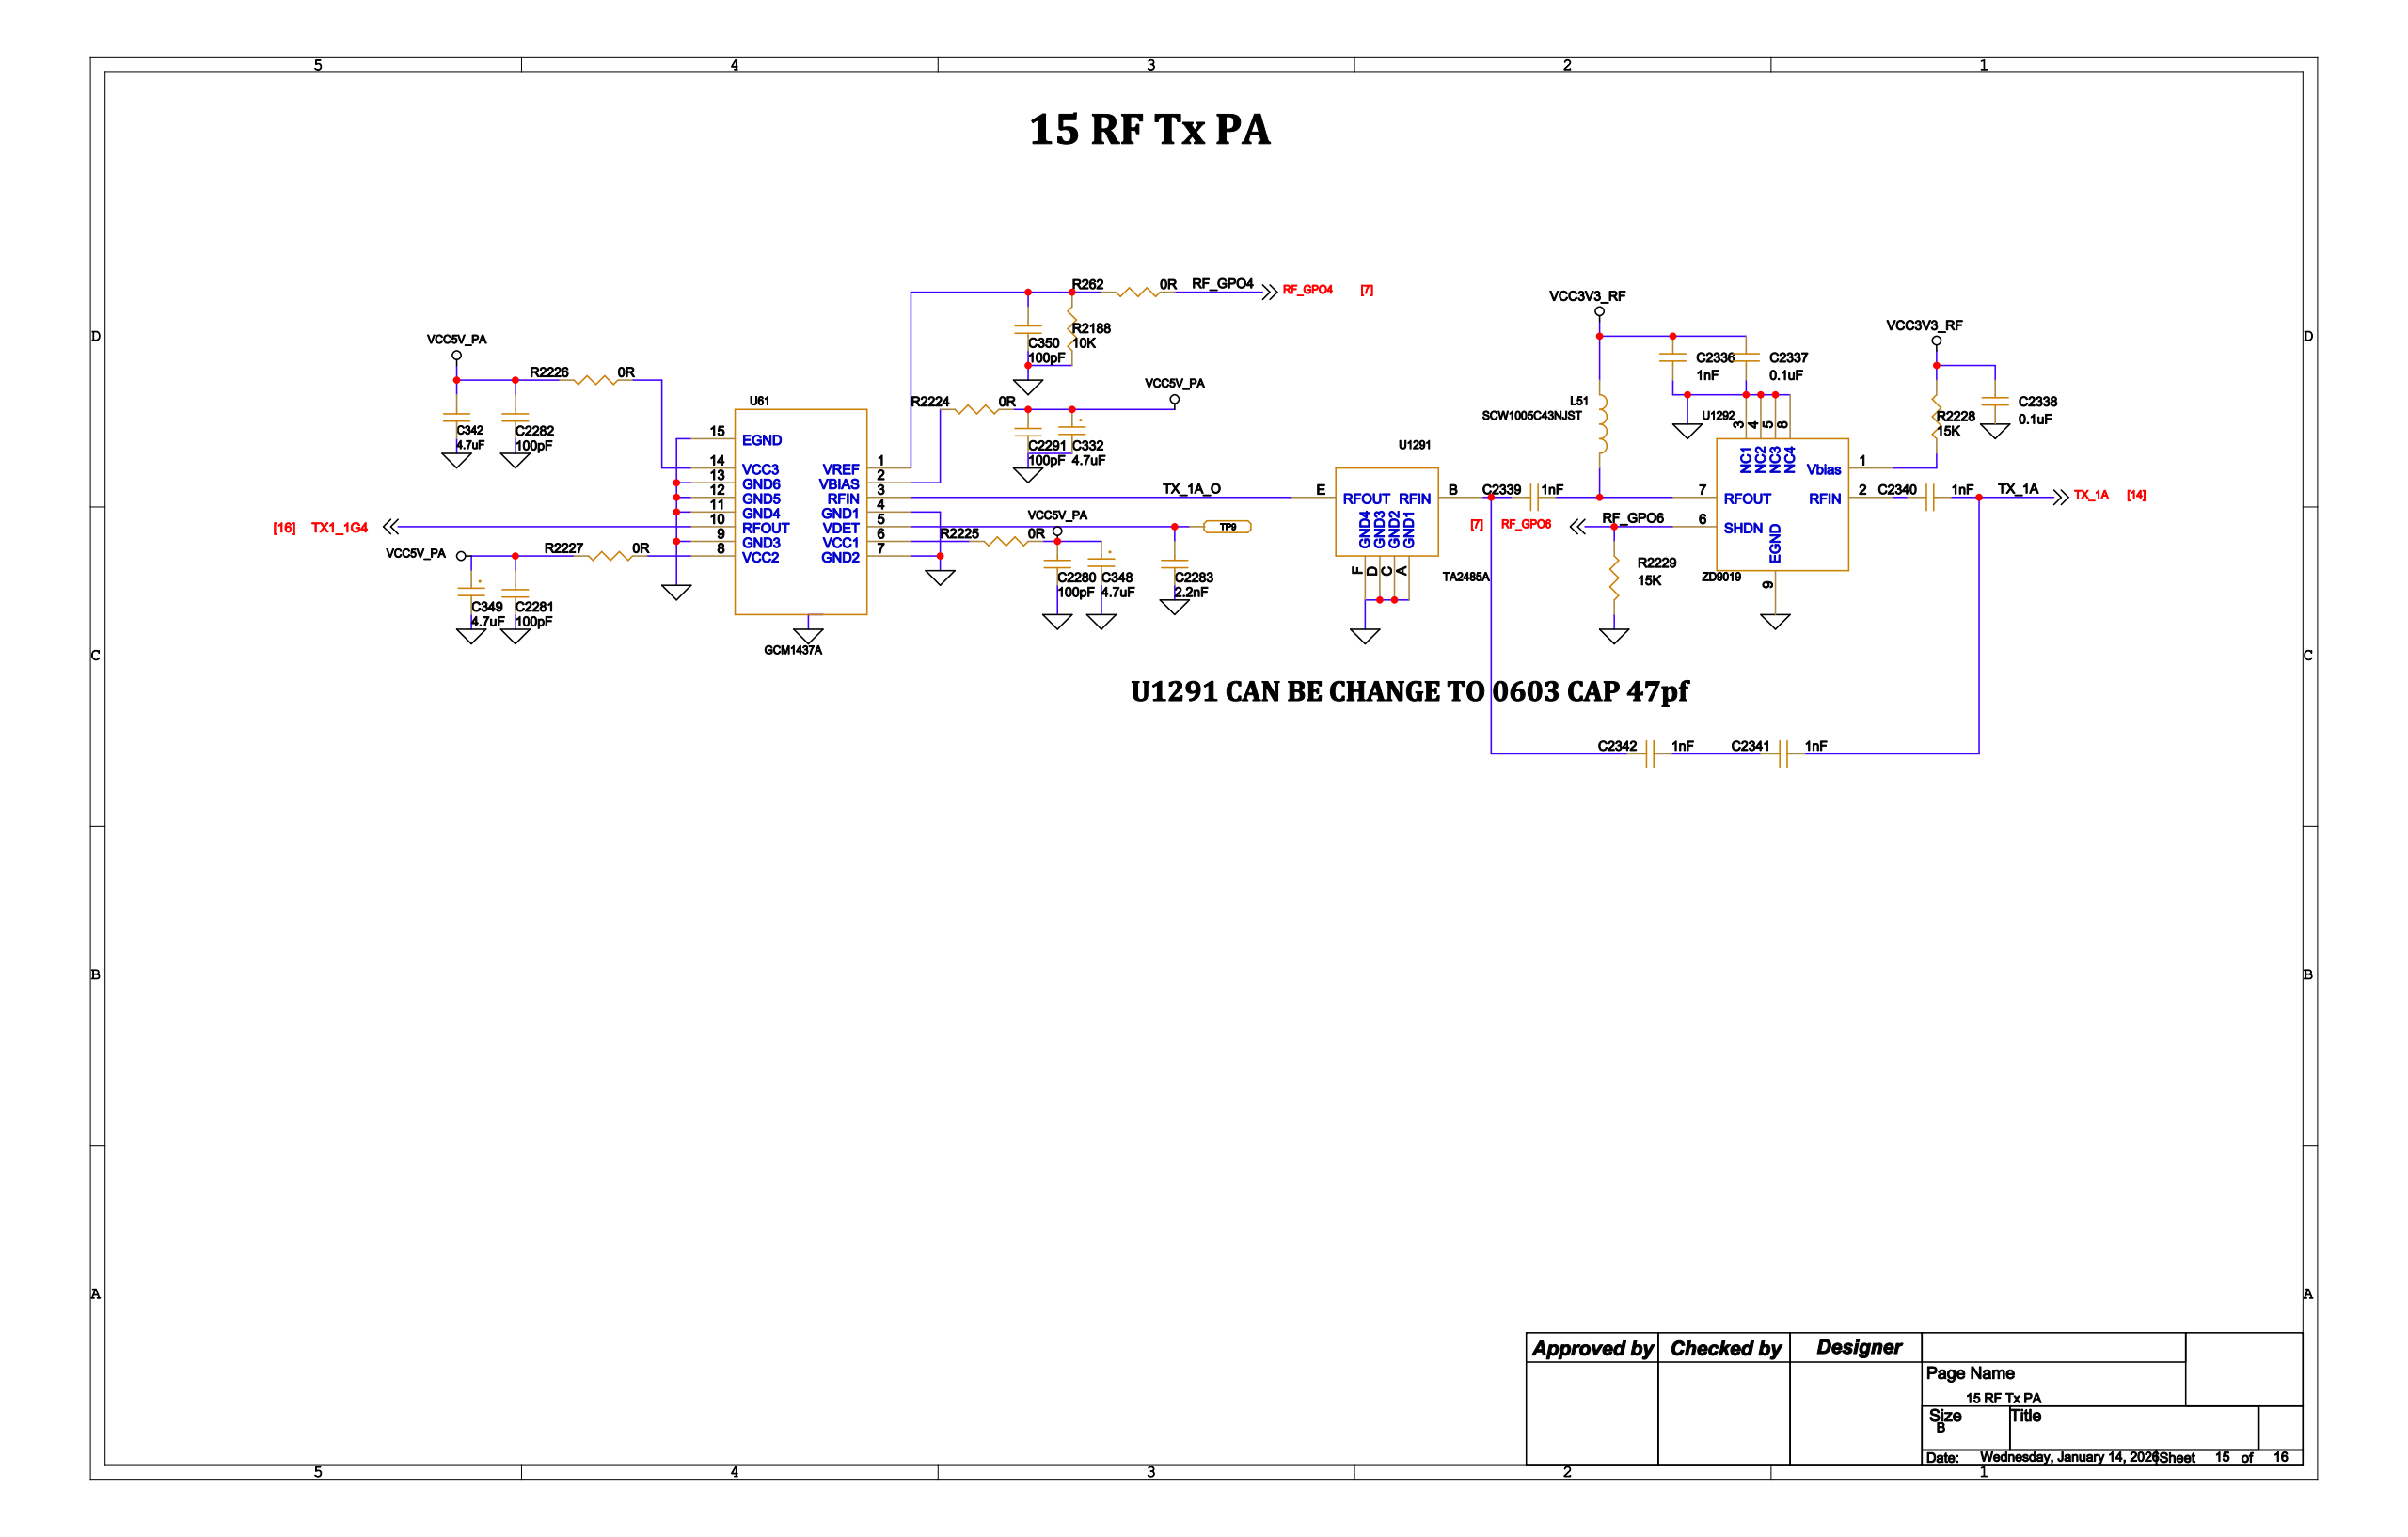Circuit board | Cadence Allegro | 442 parts | 326 nets | one sheet of the schematic
Parts on this sheet (reference | value | footprint):
C332 | 4.7uF | C0402_D
C342 | 4.7uF | C0402_D
C348 | 4.7uF | C0402_D
C349 | 4.7uF | C0402_D
C350 | 100pF | C0201
C2280 | 100pF | C0201
C2281 | 100pF | C0201
C2282 | 100pF | C0201
C2283 | 2.2nF | C0201
C2291 | 100pF | C0201
C2336 | 1nF | C0201
C2337 | 0.1uF | C0201
C2338 | 0.1uF | C0201
C2339 | 1nF | C0201
C2340 | 1nF | C0201
C2341 | 1nF | C0201
C2342 | 1nF | C0201
L51 | SCW1005C43NJST | L0201
R262 | 0R | R0201
R2188 | 10K | R0201
R2224 | 0R | R0201
R2225 | 0R | R0201
R2226 | 0R | R0201
R2227 | 0R | R0201
R2228 | 15K | R0201
R2229 | 15K | R0201
TP9 | LABTESTPOINT | LTPT28C49P
U61 | GCM1437A | PA-14-1_06-GCM1437A
U1291 | TA2485A | TA2494A
U1292 | ZD9019 | DFN2X2-8P
Nets of these parts (net: part-pin ...):
GND: C332-2 C342-1 C348-2 C349-2 C350-1 C2280-1 C2281-1 C2282-1 C2283-1 C2291-1 C2336-2 C2337-2 C2338-2 R2188-2 R2229-1 U61-4 U61-7 U61-9 U61-11 U61-12 U61-13 U61-15 U1291-A U1291-C U1291-D U1291-F U1292-3 U1292-4 U1292-5 U1292-8 U1292-9
N50595277: C2340-2 U1292-2
N50595756: C2339-1 L51-2 U1292-7
RF_GPO6: R2229-2 U1292-6
N50595497: R2228-2 U1292-1
N50309666: C2283-2 TP9-1 U61-5
VCC3V3_RF: C2336-1 C2337-1 C2338-1 L51-1 R2228-1
VCC5V_PA: C332-1 C342-2 C348-1 C349-1 C2280-2 C2281-2 C2282-2 C2291-2 R2224-2 R2225-2 R2226-1 R2227-1
N50545995: C2339-2 C2342-2 U1291-B
TX_1A_O: U61-3 U1291-E
TX1_1G4: U61-10
N50313374: R2224-1 U61-2
N50050224: R2225-1 U61-6
N50323845: R2227-2 U61-8
N50056105: R2226-2 U61-14
N49200262: C350-2 R262-1 R2188-1 U61-1
TX_1A: C2340-1 C2341-1
N50622590: C2341-2 C2342-1
RF_GPO4: R262-2